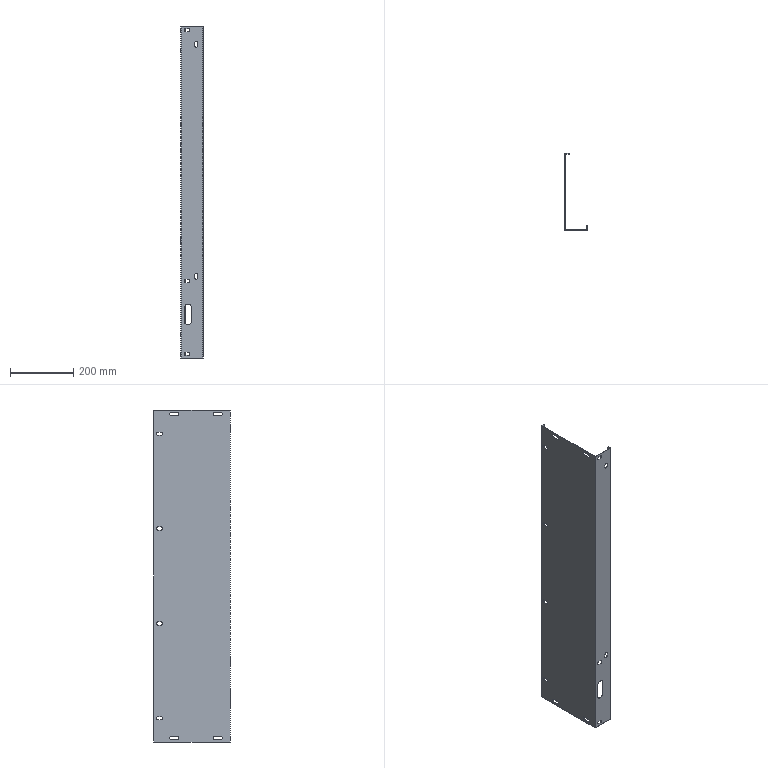Part | 1 solid | 101 faces | box 70 x 243.5 x 1050 mm | volume 422262 mm3 | plane 56 | cylinder 45 | commonest cylinder face diameters 10 x16 9 x12 11 x8 0.4 x3 2.8 x3 24 x3